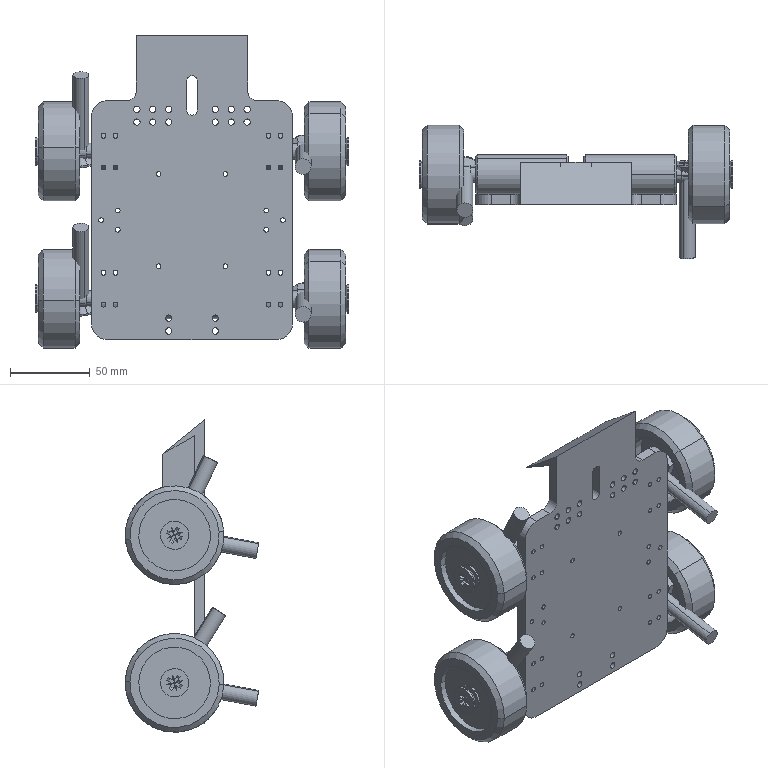Part | SolidWorks | 21 solids | 711 faces | box 196.8 x 83.824 x 196.095 mm | volume 523655 mm3 | plane 378 | cylinder 269 | cone 64 | commonest cylinder face diameters 3 x76 4 x48 0.6 x32 10 x16 17.78 x16 45 x16